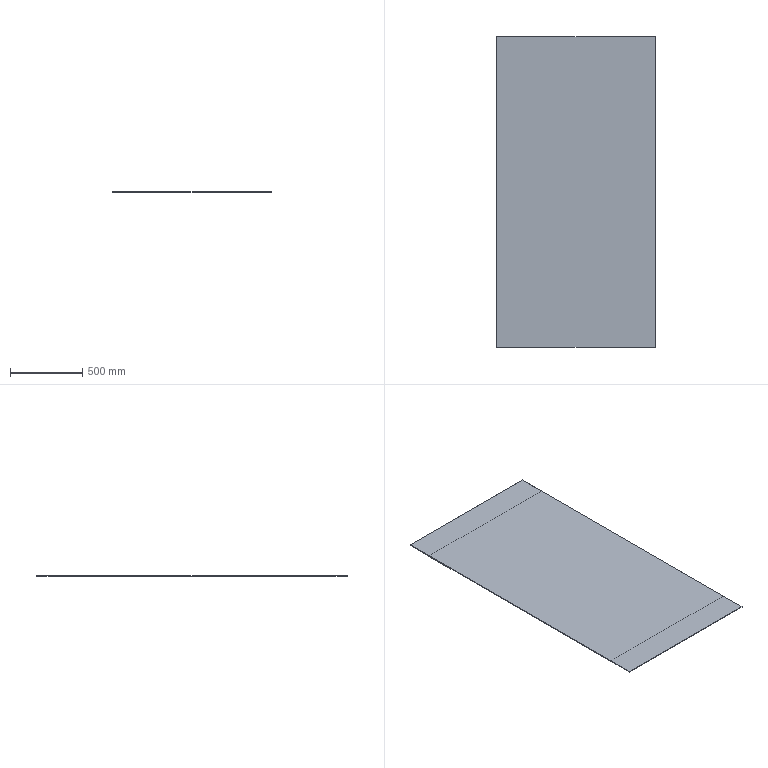Part | SolidWorks | features Extrusion 1, ICE 1 | 1 solid | 10 faces | box 1100 x 2150 x 5 mm | volume 11418000 mm3 | plane 10
STEP:
#1=CARTESIAN_POINT('',(0.,-185.,0.));
#2=VERTEX_POINT('',#1);
#3=CARTESIAN_POINT('',(1100.,-185.,0.));
#4=VERTEX_POINT('',#3);
#5=CARTESIAN_POINT('',(1100.,-185.,0.));
#6=DIRECTION('',(1.,0.,0.));
#7=VECTOR('',#6,1000.);
#8=LINE('',#5,#7);
#9=EDGE_CURVE('',#2,#4,#8,.T.);
#10=ORIENTED_EDGE('',*,*,#9,.F.);
#11=CARTESIAN_POINT('',(0.,0.,0.));
#12=VERTEX_POINT('',#11);
#13=CARTESIAN_POINT('',(0.,0.,0.));
#14=DIRECTION('',(0.,-1.,0.));
#15=VECTOR('',#14,1000.);
#16=LINE('',#13,#15);
#17=EDGE_CURVE('',#12,#2,#16,.T.);
#18=ORIENTED_EDGE('',*,*,#17,.F.);
#19=CARTESIAN_POINT('',(1100.,0.,0.));
#20=VERTEX_POINT('',#19);
#21=CARTESIAN_POINT('',(0.,0.,0.));
#22=DIRECTION('',(-1.,0.,0.));
#23=VECTOR('',#22,1000.);
#24=LINE('',#21,#23);
#25=EDGE_CURVE('',#20,#12,#24,.T.);
#26=ORIENTED_EDGE('',*,*,#25,.F.);
#27=CARTESIAN_POINT('',(1100.,0.,0.));
#28=DIRECTION('',(0.,1.,0.));
#29=VECTOR('',#28,1000.);
#30=LINE('',#27,#29);
#31=EDGE_CURVE('',#4,#20,#30,.T.);
#32=ORIENTED_EDGE('',*,*,#31,.F.);
#33=EDGE_LOOP('',(#10,#18,#26,#32));
#34=FACE_OUTER_BOUND('',#33,.T.);
#35=CARTESIAN_POINT('',(0.,0.,0.));
#36=DIRECTION('',(0.,0.,1.));
#37=DIRECTION('',(1.,0.,0.));
#38=AXIS2_PLACEMENT_3D('',#35,#36,#37);
#39=PLANE('',#38);
#40=ADVANCED_FACE('',(#34),#39,.F.);
#41=CARTESIAN_POINT('',(1100.,-1965.,0.));
#42=VERTEX_POINT('',#41);
#43=CARTESIAN_POINT('',(0.,-1965.,0.));
#44=VERTEX_POINT('',#43);
#45=CARTESIAN_POINT('',(1100.,-1965.,0.));
#46=DIRECTION('',(-1.,0.,0.));
#47=VECTOR('',#46,1000.);
#48=LINE('',#45,#47);
#49=EDGE_CURVE('',#42,#44,#48,.T.);
#50=ORIENTED_EDGE('',*,*,#49,.F.);
#51=CARTESIAN_POINT('',(1100.,-2150.,0.));
#52=VERTEX_POINT('',#51);
#53=CARTESIAN_POINT('',(1100.,0.,0.));
#54=DIRECTION('',(0.,1.,0.));
#55=VECTOR('',#54,1000.);
#56=LINE('',#53,#55);
#57=EDGE_CURVE('',#52,#42,#56,.T.);
#58=ORIENTED_EDGE('',*,*,#57,.F.);
#59=CARTESIAN_POINT('',(0.,-2150.,0.));
#60=VERTEX_POINT('',#59);
#61=CARTESIAN_POINT('',(0.,-2150.,0.));
#62=DIRECTION('',(1.,0.,0.));
#63=VECTOR('',#62,1000.);
#64=LINE('',#61,#63);
#65=EDGE_CURVE('',#60,#52,#64,.T.);
#66=ORIENTED_EDGE('',*,*,#65,.F.);
#67=CARTESIAN_POINT('',(0.,0.,0.));
#68=DIRECTION('',(0.,-1.,0.));
#69=VECTOR('',#68,1000.);
#70=LINE('',#67,#69);
#71=EDGE_CURVE('',#44,#60,#70,.T.);
#72=ORIENTED_EDGE('',*,*,#71,.F.);
#73=EDGE_LOOP('',(#50,#58,#66,#72));
#74=FACE_OUTER_BOUND('',#73,.T.);
#75=CARTESIAN_POINT('',(0.,0.,0.));
#76=DIRECTION('',(0.,0.,1.));
#77=DIRECTION('',(1.,0.,0.));
#78=AXIS2_PLACEMENT_3D('',#75,#76,#77);
#79=PLANE('',#78);
#80=ADVANCED_FACE('',(#74),#79,.F.);
#81=ORIENTED_EDGE('',*,*,#17,.T.);
#82=CARTESIAN_POINT('',(0.,-185.,-1.));
#83=VERTEX_POINT('',#82);
#84=CARTESIAN_POINT('',(0.,-185.,-1.));
#85=DIRECTION('',(0.,0.,1.));
#86=VECTOR('',#85,1000.);
#87=LINE('',#84,#86);
#88=EDGE_CURVE('',#83,#2,#87,.T.);
#89=ORIENTED_EDGE('',*,*,#88,.F.);
#90=CARTESIAN_POINT('',(0.,-1965.,-1.));
#91=VERTEX_POINT('',#90);
#92=CARTESIAN_POINT('',(0.,-1965.,-1.));
#93=DIRECTION('',(0.,1.,0.));
#94=VECTOR('',#93,1000.);
#95=LINE('',#92,#94);
#96=EDGE_CURVE('',#91,#83,#95,.T.);
#97=ORIENTED_EDGE('',*,*,#96,.F.);
#98=CARTESIAN_POINT('',(0.,-1965.,-1.));
#99=DIRECTION('',(0.,0.,1.));
#100=VECTOR('',#99,1000.);
#101=LINE('',#98,#100);
#102=EDGE_CURVE('',#91,#44,#101,.T.);
#103=ORIENTED_EDGE('',*,*,#102,.T.);
#104=ORIENTED_EDGE('',*,*,#71,.T.);
#105=CARTESIAN_POINT('',(0.,-2150.,4.));
#106=VERTEX_POINT('',#105);
#107=CARTESIAN_POINT('',(0.,-2150.,4.));
#108=DIRECTION('',(0.,0.,-1.));
#109=VECTOR('',#108,1000.);
#110=LINE('',#107,#109);
#111=EDGE_CURVE('',#106,#60,#110,.T.);
#112=ORIENTED_EDGE('',*,*,#111,.F.);
#113=CARTESIAN_POINT('',(0.,0.,4.));
#114=VERTEX_POINT('',#113);
#115=CARTESIAN_POINT('',(0.,0.,4.));
#116=DIRECTION('',(0.,-1.,0.));
#117=VECTOR('',#116,1000.);
#118=LINE('',#115,#117);
#119=EDGE_CURVE('',#114,#106,#118,.T.);
#120=ORIENTED_EDGE('',*,*,#119,.F.);
#121=CARTESIAN_POINT('',(0.,0.,4.));
#122=DIRECTION('',(0.,0.,-1.));
#123=VECTOR('',#122,1000.);
#124=LINE('',#121,#123);
#125=EDGE_CURVE('',#114,#12,#124,.T.);
#126=ORIENTED_EDGE('',*,*,#125,.T.);
#127=EDGE_LOOP('',(#81,#89,#97,#103,#104,#112,#120,#126));
#128=FACE_OUTER_BOUND('',#127,.T.);
#129=CARTESIAN_POINT('',(0.,0.,4.));
#130=DIRECTION('',(1.,0.,0.));
#131=DIRECTION('',(0.,1.,0.));
#132=AXIS2_PLACEMENT_3D('',#129,#130,#131);
#133=PLANE('',#132);
#134=ADVANCED_FACE('',(#128),#133,.F.);
#135=ORIENTED_EDGE('',*,*,#65,.T.);
#136=CARTESIAN_POINT('',(1100.,-2150.,4.));
#137=VERTEX_POINT('',#136);
#138=CARTESIAN_POINT('',(1100.,-2150.,4.));
#139=DIRECTION('',(0.,0.,-1.));
#140=VECTOR('',#139,1000.);
#141=LINE('',#138,#140);
#142=EDGE_CURVE('',#137,#52,#141,.T.);
#143=ORIENTED_EDGE('',*,*,#142,.F.);
#144=CARTESIAN_POINT('',(0.,-2150.,4.));
#145=DIRECTION('',(1.,0.,0.));
#146=VECTOR('',#145,1000.);
#147=LINE('',#144,#146);
#148=EDGE_CURVE('',#106,#137,#147,.T.);
#149=ORIENTED_EDGE('',*,*,#148,.F.);
#150=ORIENTED_EDGE('',*,*,#111,.T.);
#151=EDGE_LOOP('',(#135,#143,#149,#150));
#152=FACE_OUTER_BOUND('',#151,.T.);
#153=CARTESIAN_POINT('',(0.,-2150.,4.));
#154=DIRECTION('',(0.,1.,0.));
#155=DIRECTION('',(0.,0.,1.));
#156=AXIS2_PLACEMENT_3D('',#153,#154,#155);
#157=PLANE('',#156);
#158=ADVANCED_FACE('',(#152),#157,.F.);
#159=ORIENTED_EDGE('',*,*,#57,.T.);
#160=CARTESIAN_POINT('',(1100.,-1965.,-1.));
#161=VERTEX_POINT('',#160);
#162=CARTESIAN_POINT('',(1100.,-1965.,-1.));
#163=DIRECTION('',(0.,0.,1.));
#164=VECTOR('',#163,1000.);
#165=LINE('',#162,#164);
#166=EDGE_CURVE('',#161,#42,#165,.T.);
#167=ORIENTED_EDGE('',*,*,#166,.F.);
#168=CARTESIAN_POINT('',(1100.,-185.,-1.));
#169=VERTEX_POINT('',#168);
#170=CARTESIAN_POINT('',(1100.,-1965.,-1.));
#171=DIRECTION('',(0.,-1.,0.));
#172=VECTOR('',#171,1000.);
#173=LINE('',#170,#172);
#174=EDGE_CURVE('',#169,#161,#173,.T.);
#175=ORIENTED_EDGE('',*,*,#174,.F.);
#176=CARTESIAN_POINT('',(1100.,-185.,-1.));
#177=DIRECTION('',(0.,0.,1.));
#178=VECTOR('',#177,1000.);
#179=LINE('',#176,#178);
#180=EDGE_CURVE('',#169,#4,#179,.T.);
#181=ORIENTED_EDGE('',*,*,#180,.T.);
#182=ORIENTED_EDGE('',*,*,#31,.T.);
#183=CARTESIAN_POINT('',(1100.,0.,4.));
#184=VERTEX_POINT('',#183);
#185=CARTESIAN_POINT('',(1100.,0.,4.));
#186=DIRECTION('',(0.,0.,-1.));
#187=VECTOR('',#186,1000.);
#188=LINE('',#185,#187);
#189=EDGE_CURVE('',#184,#20,#188,.T.);
#190=ORIENTED_EDGE('',*,*,#189,.F.);
#191=CARTESIAN_POINT('',(1100.,0.,4.));
#192=DIRECTION('',(0.,1.,0.));
#193=VECTOR('',#192,1000.);
#194=LINE('',#191,#193);
#195=EDGE_CURVE('',#137,#184,#194,.T.);
#196=ORIENTED_EDGE('',*,*,#195,.F.);
#197=ORIENTED_EDGE('',*,*,#142,.T.);
#198=EDGE_LOOP('',(#159,#167,#175,#181,#182,#190,#196,#197));
#199=FACE_OUTER_BOUND('',#198,.T.);
#200=CARTESIAN_POINT('',(1100.,0.,4.));
#201=DIRECTION('',(-1.,0.,0.));
#202=DIRECTION('',(0.,0.,1.));
#203=AXIS2_PLACEMENT_3D('',#200,#201,#202);
#204=PLANE('',#203);
#205=ADVANCED_FACE('',(#199),#204,.F.);
#206=ORIENTED_EDGE('',*,*,#25,.T.);
#207=ORIENTED_EDGE('',*,*,#125,.F.);
#208=CARTESIAN_POINT('',(0.,0.,4.));
#209=DIRECTION('',(-1.,0.,0.));
#210=VECTOR('',#209,1000.);
#211=LINE('',#208,#210);
#212=EDGE_CURVE('',#184,#114,#211,.T.);
#213=ORIENTED_EDGE('',*,*,#212,.F.);
#214=ORIENTED_EDGE('',*,*,#189,.T.);
#215=EDGE_LOOP('',(#206,#207,#213,#214));
#216=FACE_OUTER_BOUND('',#215,.T.);
#217=CARTESIAN_POINT('',(0.,0.,4.));
#218=DIRECTION('',(0.,-1.,0.));
#219=DIRECTION('',(0.,0.,-1.));
#220=AXIS2_PLACEMENT_3D('',#217,#218,#219);
#221=PLANE('',#220);
#222=ADVANCED_FACE('',(#216),#221,.F.);
#223=ORIENTED_EDGE('',*,*,#119,.T.);
#224=ORIENTED_EDGE('',*,*,#148,.T.);
#225=ORIENTED_EDGE('',*,*,#195,.T.);
#226=ORIENTED_EDGE('',*,*,#212,.T.);
#227=EDGE_LOOP('',(#223,#224,#225,#226));
#228=FACE_OUTER_BOUND('',#227,.T.);
#229=CARTESIAN_POINT('',(0.,0.,4.));
#230=DIRECTION('',(0.,0.,1.));
#231=DIRECTION('',(1.,0.,0.));
#232=AXIS2_PLACEMENT_3D('',#229,#230,#231);
#233=PLANE('',#232);
#234=ADVANCED_FACE('',(#228),#233,.T.);
#235=ORIENTED_EDGE('',*,*,#49,.T.);
#236=ORIENTED_EDGE('',*,*,#102,.F.);
#237=CARTESIAN_POINT('',(1100.,-1965.,-1.));
#238=DIRECTION('',(-1.,0.,0.));
#239=VECTOR('',#238,1000.);
#240=LINE('',#237,#239);
#241=EDGE_CURVE('',#161,#91,#240,.T.);
#242=ORIENTED_EDGE('',*,*,#241,.F.);
#243=ORIENTED_EDGE('',*,*,#166,.T.);
#244=EDGE_LOOP('',(#235,#236,#242,#243));
#245=FACE_OUTER_BOUND('',#244,.T.);
#246=CARTESIAN_POINT('',(1100.,-1965.,-1.));
#247=DIRECTION('',(0.,1.,0.));
#248=DIRECTION('',(0.,0.,1.));
#249=AXIS2_PLACEMENT_3D('',#246,#247,#248);
#250=PLANE('',#249);
#251=ADVANCED_FACE('',(#245),#250,.F.);
#252=ORIENTED_EDGE('',*,*,#9,.T.);
#253=ORIENTED_EDGE('',*,*,#180,.F.);
#254=CARTESIAN_POINT('',(1100.,-185.,-1.));
#255=DIRECTION('',(1.,0.,0.));
#256=VECTOR('',#255,1000.);
#257=LINE('',#254,#256);
#258=EDGE_CURVE('',#83,#169,#257,.T.);
#259=ORIENTED_EDGE('',*,*,#258,.F.);
#260=ORIENTED_EDGE('',*,*,#88,.T.);
#261=EDGE_LOOP('',(#252,#253,#259,#260));
#262=FACE_OUTER_BOUND('',#261,.T.);
#263=CARTESIAN_POINT('',(1100.,-185.,-1.));
#264=DIRECTION('',(0.,-1.,0.));
#265=DIRECTION('',(0.,0.,-1.));
#266=AXIS2_PLACEMENT_3D('',#263,#264,#265);
#267=PLANE('',#266);
#268=ADVANCED_FACE('',(#262),#267,.F.);
#269=ORIENTED_EDGE('',*,*,#174,.T.);
#270=ORIENTED_EDGE('',*,*,#241,.T.);
#271=ORIENTED_EDGE('',*,*,#96,.T.);
#272=ORIENTED_EDGE('',*,*,#258,.T.);
#273=EDGE_LOOP('',(#269,#270,#271,#272));
#274=FACE_OUTER_BOUND('',#273,.T.);
#275=CARTESIAN_POINT('',(0.,0.,-1.));
#276=DIRECTION('',(0.,0.,1.));
#277=DIRECTION('',(1.,0.,0.));
#278=AXIS2_PLACEMENT_3D('',#275,#276,#277);
#279=PLANE('',#278);
#280=ADVANCED_FACE('',(#274),#279,.F.);
#281=CLOSED_SHELL('',(#40,#80,#134,#158,#205,#222,#234,#251,#268,#280));
#282=MANIFOLD_SOLID_BREP('',#281);
#283=CARTESIAN_POINT('',(0.,0.,0.));
#284=DIRECTION('',(0.,0.,1.));
#285=DIRECTION('',(1.,0.,0.));
#286=AXIS2_PLACEMENT_3D('',#283,#284,#285);
#287=(LENGTH_UNIT()NAMED_UNIT(*)SI_UNIT(.MILLI.,.METRE.));
#288=UNCERTAINTY_MEASURE_WITH_UNIT(LENGTH_MEASURE(0.00001),#287,'','');
#289=(NAMED_UNIT(*)PLANE_ANGLE_UNIT()SI_UNIT($,.RADIAN.));
#290=(NAMED_UNIT(*)SI_UNIT($,.STERADIAN.)SOLID_ANGLE_UNIT());
#291=(GEOMETRIC_REPRESENTATION_CONTEXT(3)GLOBAL_UNCERTAINTY_ASSIGNED_CONTEXT((#288))GLOBAL_UNIT_ASSIGNED_CONTEXT((#287,#289,#290))REPRESENTATION_CONTEXT('',''));
#292=ADVANCED_BREP_SHAPE_REPRESENTATION('',(#282,#286),#291);